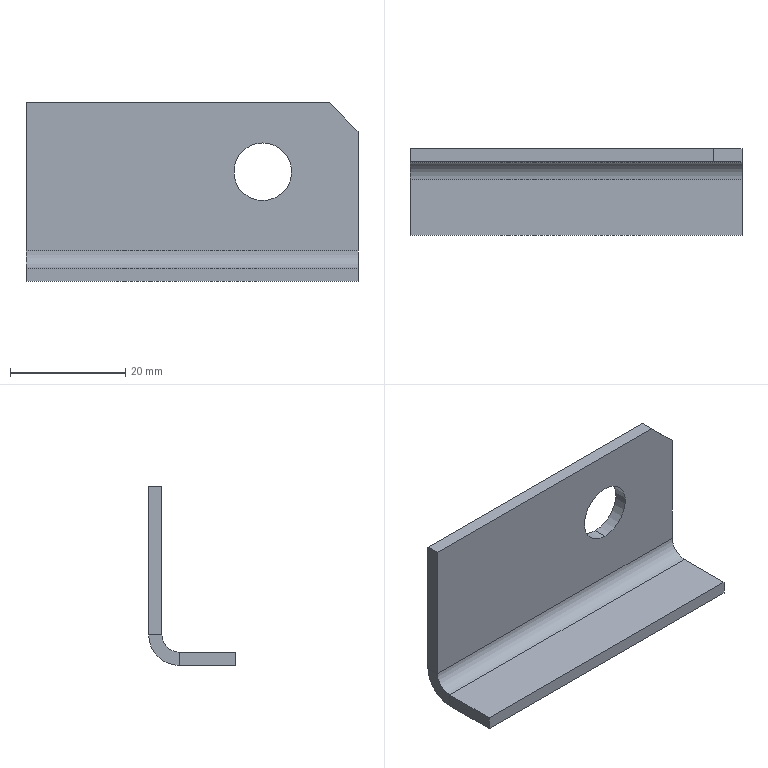Part | SolidWorks | features Chamfer 1, FlatPattern 1, ICE 1, SMBaseFlange 1, SheetMetal 1 | 1 solid | 17 faces | box 57.5 x 15 x 31 mm | volume 5334 mm3 | plane 13 | cylinder 4 | commonest cylinder face diameters 10 x2 6 x1 10.6 x1
STEP:
#1=CARTESIAN_POINT('',(12.25,15.,14.));
#2=VERTEX_POINT('',#1);
#3=CARTESIAN_POINT('',(12.25,15.,24.));
#4=VERTEX_POINT('',#3);
#5=CARTESIAN_POINT('',(12.25,15.,19.));
#6=DIRECTION('',(0.,1.,0.));
#7=DIRECTION('',(0.,0.,-1.));
#8=AXIS2_PLACEMENT_3D('',#5,#6,#7);
#9=CIRCLE('',#8,5.);
#10=EDGE_CURVE('',#2,#4,#9,.T.);
#11=ORIENTED_EDGE('',*,*,#10,.T.);
#12=CARTESIAN_POINT('',(12.25,12.7,24.));
#13=VERTEX_POINT('',#12);
#14=CARTESIAN_POINT('',(12.25,15.001,24.));
#15=DIRECTION('',(0.,-1.,0.));
#16=VECTOR('',#15,1000.);
#17=LINE('',#14,#16);
#18=EDGE_CURVE('',#4,#13,#17,.T.);
#19=ORIENTED_EDGE('',*,*,#18,.T.);
#20=CARTESIAN_POINT('',(12.25,12.7,14.));
#21=VERTEX_POINT('',#20);
#22=CARTESIAN_POINT('',(12.25,12.7,19.));
#23=DIRECTION('',(0.,-1.,0.));
#24=DIRECTION('',(0.,0.,-1.));
#25=AXIS2_PLACEMENT_3D('',#22,#23,#24);
#26=CIRCLE('',#25,5.);
#27=EDGE_CURVE('',#13,#21,#26,.T.);
#28=ORIENTED_EDGE('',*,*,#27,.T.);
#29=CARTESIAN_POINT('',(12.25,15.001,14.));
#30=DIRECTION('',(0.,-1.,0.));
#31=VECTOR('',#30,1000.);
#32=LINE('',#29,#31);
#33=EDGE_CURVE('',#2,#21,#32,.T.);
#34=ORIENTED_EDGE('',*,*,#33,.F.);
#35=EDGE_LOOP('',(#11,#19,#28,#34));
#36=FACE_OUTER_BOUND('',#35,.T.);
#37=CARTESIAN_POINT('',(12.25,15.001,19.));
#38=DIRECTION('',(0.,-1.,0.));
#39=DIRECTION('',(0.,0.,-1.));
#40=AXIS2_PLACEMENT_3D('',#37,#38,#39);
#41=CYLINDRICAL_SURFACE('',#40,5.);
#42=ADVANCED_FACE('',(#36),#41,.F.);
#43=CARTESIAN_POINT('',(28.75,9.7,0.));
#44=VERTEX_POINT('',#43);
#45=CARTESIAN_POINT('',(28.75,9.7,2.3));
#46=VERTEX_POINT('',#45);
#47=CARTESIAN_POINT('',(28.75,9.7,0.));
#48=DIRECTION('',(0.,0.,1.));
#49=VECTOR('',#48,1000.);
#50=LINE('',#47,#49);
#51=EDGE_CURVE('',#44,#46,#50,.T.);
#52=ORIENTED_EDGE('',*,*,#51,.F.);
#53=CARTESIAN_POINT('',(28.75,15.,5.3));
#54=VERTEX_POINT('',#53);
#55=CARTESIAN_POINT('',(28.75,9.7,5.3));
#56=DIRECTION('',(1.,0.,0.));
#57=DIRECTION('',(0.,0.,1.));
#58=AXIS2_PLACEMENT_3D('',#55,#56,#57);
#59=CIRCLE('',#58,5.3);
#60=EDGE_CURVE('',#44,#54,#59,.T.);
#61=ORIENTED_EDGE('',*,*,#60,.T.);
#62=CARTESIAN_POINT('',(28.75,12.7,5.3));
#63=VERTEX_POINT('',#62);
#64=CARTESIAN_POINT('',(28.75,12.7,5.3));
#65=DIRECTION('',(0.,1.,0.));
#66=VECTOR('',#65,1000.);
#67=LINE('',#64,#66);
#68=EDGE_CURVE('',#63,#54,#67,.T.);
#69=ORIENTED_EDGE('',*,*,#68,.F.);
#70=CARTESIAN_POINT('',(28.75,9.7,5.3));
#71=DIRECTION('',(1.,0.,0.));
#72=DIRECTION('',(0.,0.,-1.));
#73=AXIS2_PLACEMENT_3D('',#70,#71,#72);
#74=CIRCLE('',#73,3.);
#75=EDGE_CURVE('',#46,#63,#74,.T.);
#76=ORIENTED_EDGE('',*,*,#75,.F.);
#77=EDGE_LOOP('',(#52,#61,#69,#76));
#78=FACE_OUTER_BOUND('',#77,.T.);
#79=CARTESIAN_POINT('',(28.75,9.7,0.));
#80=DIRECTION('',(1.,0.,0.));
#81=DIRECTION('',(0.,0.,-1.));
#82=AXIS2_PLACEMENT_3D('',#79,#80,#81);
#83=PLANE('',#82);
#84=ADVANCED_FACE('',(#78),#83,.T.);
#85=CARTESIAN_POINT('',(28.75,0.,0.));
#86=VERTEX_POINT('',#85);
#87=CARTESIAN_POINT('',(28.75,0.,0.));
#88=DIRECTION('',(0.,1.,0.));
#89=VECTOR('',#88,1000.);
#90=LINE('',#87,#89);
#91=EDGE_CURVE('',#86,#44,#90,.T.);
#92=ORIENTED_EDGE('',*,*,#91,.T.);
#93=ORIENTED_EDGE('',*,*,#51,.T.);
#94=CARTESIAN_POINT('',(28.75,0.,2.3));
#95=VERTEX_POINT('',#94);
#96=CARTESIAN_POINT('',(28.75,0.,2.3));
#97=DIRECTION('',(0.,1.,0.));
#98=VECTOR('',#97,1000.);
#99=LINE('',#96,#98);
#100=EDGE_CURVE('',#95,#46,#99,.T.);
#101=ORIENTED_EDGE('',*,*,#100,.F.);
#102=CARTESIAN_POINT('',(28.75,0.,0.));
#103=DIRECTION('',(0.,0.,1.));
#104=VECTOR('',#103,1000.);
#105=LINE('',#102,#104);
#106=EDGE_CURVE('',#86,#95,#105,.T.);
#107=ORIENTED_EDGE('',*,*,#106,.F.);
#108=EDGE_LOOP('',(#92,#93,#101,#107));
#109=FACE_OUTER_BOUND('',#108,.T.);
#110=CARTESIAN_POINT('',(28.75,12.7,5.3));
#111=DIRECTION('',(1.,0.,0.));
#112=DIRECTION('',(0.,0.,-1.));
#113=AXIS2_PLACEMENT_3D('',#110,#111,#112);
#114=PLANE('',#113);
#115=ADVANCED_FACE('',(#109),#114,.T.);
#116=CARTESIAN_POINT('',(-28.75,15.,5.3));
#117=VERTEX_POINT('',#116);
#118=CARTESIAN_POINT('',(-28.75,12.7,5.3));
#119=VERTEX_POINT('',#118);
#120=CARTESIAN_POINT('',(-28.75,15.,5.3));
#121=DIRECTION('',(0.,-1.,0.));
#122=VECTOR('',#121,1000.);
#123=LINE('',#120,#122);
#124=EDGE_CURVE('',#117,#119,#123,.T.);
#125=ORIENTED_EDGE('',*,*,#124,.F.);
#126=CARTESIAN_POINT('',(-28.75,9.7,0.));
#127=VERTEX_POINT('',#126);
#128=CARTESIAN_POINT('',(-28.75,9.7,5.3));
#129=DIRECTION('',(1.,0.,0.));
#130=DIRECTION('',(0.,0.,1.));
#131=AXIS2_PLACEMENT_3D('',#128,#129,#130);
#132=CIRCLE('',#131,5.3);
#133=EDGE_CURVE('',#127,#117,#132,.T.);
#134=ORIENTED_EDGE('',*,*,#133,.F.);
#135=CARTESIAN_POINT('',(-28.75,9.7,2.3));
#136=VERTEX_POINT('',#135);
#137=CARTESIAN_POINT('',(-28.75,9.7,2.3));
#138=DIRECTION('',(0.,0.,-1.));
#139=VECTOR('',#138,1000.);
#140=LINE('',#137,#139);
#141=EDGE_CURVE('',#136,#127,#140,.T.);
#142=ORIENTED_EDGE('',*,*,#141,.F.);
#143=CARTESIAN_POINT('',(-28.75,9.7,5.3));
#144=DIRECTION('',(1.,0.,0.));
#145=DIRECTION('',(0.,0.,-1.));
#146=AXIS2_PLACEMENT_3D('',#143,#144,#145);
#147=CIRCLE('',#146,3.);
#148=EDGE_CURVE('',#136,#119,#147,.T.);
#149=ORIENTED_EDGE('',*,*,#148,.T.);
#150=EDGE_LOOP('',(#125,#134,#142,#149));
#151=FACE_OUTER_BOUND('',#150,.T.);
#152=CARTESIAN_POINT('',(-28.75,15.,5.3));
#153=DIRECTION('',(-1.,0.,0.));
#154=DIRECTION('',(0.,0.,1.));
#155=AXIS2_PLACEMENT_3D('',#152,#153,#154);
#156=PLANE('',#155);
#157=ADVANCED_FACE('',(#151),#156,.T.);
#158=CARTESIAN_POINT('',(-28.75,15.,31.));
#159=VERTEX_POINT('',#158);
#160=CARTESIAN_POINT('',(-28.75,15.,0.));
#161=DIRECTION('',(0.,0.,1.));
#162=VECTOR('',#161,1000.);
#163=LINE('',#160,#162);
#164=EDGE_CURVE('',#117,#159,#163,.T.);
#165=ORIENTED_EDGE('',*,*,#164,.F.);
#166=ORIENTED_EDGE('',*,*,#124,.T.);
#167=CARTESIAN_POINT('',(-28.75,12.7,31.));
#168=VERTEX_POINT('',#167);
#169=CARTESIAN_POINT('',(-28.75,12.7,0.));
#170=DIRECTION('',(0.,0.,1.));
#171=VECTOR('',#170,1000.);
#172=LINE('',#169,#171);
#173=EDGE_CURVE('',#119,#168,#172,.T.);
#174=ORIENTED_EDGE('',*,*,#173,.T.);
#175=CARTESIAN_POINT('',(-28.75,12.7,31.));
#176=DIRECTION('',(0.,1.,0.));
#177=VECTOR('',#176,1000.);
#178=LINE('',#175,#177);
#179=EDGE_CURVE('',#168,#159,#178,.T.);
#180=ORIENTED_EDGE('',*,*,#179,.T.);
#181=EDGE_LOOP('',(#165,#166,#174,#180));
#182=FACE_OUTER_BOUND('',#181,.T.);
#183=CARTESIAN_POINT('',(-28.75,9.7,2.3));
#184=DIRECTION('',(-1.,0.,0.));
#185=DIRECTION('',(0.,0.,1.));
#186=AXIS2_PLACEMENT_3D('',#183,#184,#185);
#187=PLANE('',#186);
#188=ADVANCED_FACE('',(#182),#187,.T.);
#189=ORIENTED_EDGE('',*,*,#10,.F.);
#190=CARTESIAN_POINT('',(12.25,15.,19.));
#191=DIRECTION('',(0.,1.,0.));
#192=DIRECTION('',(0.,0.,-1.));
#193=AXIS2_PLACEMENT_3D('',#190,#191,#192);
#194=CIRCLE('',#193,5.);
#195=EDGE_CURVE('',#4,#2,#194,.T.);
#196=ORIENTED_EDGE('',*,*,#195,.F.);
#197=EDGE_LOOP('',(#189,#196));
#198=FACE_BOUND('',#197,.T.);
#199=CARTESIAN_POINT('',(23.75,15.,31.));
#200=VERTEX_POINT('',#199);
#201=CARTESIAN_POINT('',(28.75,15.,31.));
#202=DIRECTION('',(-1.,0.,0.));
#203=VECTOR('',#202,1000.);
#204=LINE('',#201,#203);
#205=EDGE_CURVE('',#200,#159,#204,.T.);
#206=ORIENTED_EDGE('',*,*,#205,.F.);
#207=CARTESIAN_POINT('',(28.75,15.,26.));
#208=VERTEX_POINT('',#207);
#209=CARTESIAN_POINT('',(23.75,15.,31.));
#210=DIRECTION('',(0.7071,0.,-0.7071));
#211=VECTOR('',#210,1000.);
#212=LINE('',#209,#211);
#213=EDGE_CURVE('',#200,#208,#212,.T.);
#214=ORIENTED_EDGE('',*,*,#213,.T.);
#215=CARTESIAN_POINT('',(28.75,15.,0.));
#216=DIRECTION('',(0.,0.,1.));
#217=VECTOR('',#216,1000.);
#218=LINE('',#215,#217);
#219=EDGE_CURVE('',#54,#208,#218,.T.);
#220=ORIENTED_EDGE('',*,*,#219,.F.);
#221=CARTESIAN_POINT('',(28.75,15.,5.3));
#222=DIRECTION('',(-1.,0.,0.));
#223=VECTOR('',#222,1000.);
#224=LINE('',#221,#223);
#225=EDGE_CURVE('',#54,#117,#224,.T.);
#226=ORIENTED_EDGE('',*,*,#225,.T.);
#227=ORIENTED_EDGE('',*,*,#164,.T.);
#228=EDGE_LOOP('',(#206,#214,#220,#226,#227));
#229=FACE_OUTER_BOUND('',#228,.T.);
#230=CARTESIAN_POINT('',(28.75,15.,0.));
#231=DIRECTION('',(0.,-1.,0.));
#232=DIRECTION('',(0.,0.,-1.));
#233=AXIS2_PLACEMENT_3D('',#230,#231,#232);
#234=PLANE('',#233);
#235=ADVANCED_FACE('',(#198,#229),#234,.F.);
#236=CARTESIAN_POINT('',(23.75,12.7,31.));
#237=VERTEX_POINT('',#236);
#238=CARTESIAN_POINT('',(28.75,12.7,31.));
#239=DIRECTION('',(-1.,0.,0.));
#240=VECTOR('',#239,1000.);
#241=LINE('',#238,#240);
#242=EDGE_CURVE('',#237,#168,#241,.T.);
#243=ORIENTED_EDGE('',*,*,#242,.F.);
#244=CARTESIAN_POINT('',(23.75,12.7,31.));
#245=DIRECTION('',(0.,1.,0.));
#246=VECTOR('',#245,1000.);
#247=LINE('',#244,#246);
#248=EDGE_CURVE('',#237,#200,#247,.T.);
#249=ORIENTED_EDGE('',*,*,#248,.T.);
#250=ORIENTED_EDGE('',*,*,#205,.T.);
#251=ORIENTED_EDGE('',*,*,#179,.F.);
#252=EDGE_LOOP('',(#243,#249,#250,#251));
#253=FACE_OUTER_BOUND('',#252,.T.);
#254=CARTESIAN_POINT('',(28.75,12.7,31.));
#255=DIRECTION('',(0.,0.,1.));
#256=DIRECTION('',(1.,0.,0.));
#257=AXIS2_PLACEMENT_3D('',#254,#255,#256);
#258=PLANE('',#257);
#259=ADVANCED_FACE('',(#253),#258,.T.);
#260=CARTESIAN_POINT('',(12.25,12.7,19.));
#261=DIRECTION('',(0.,-1.,0.));
#262=DIRECTION('',(0.,0.,-1.));
#263=AXIS2_PLACEMENT_3D('',#260,#261,#262);
#264=CIRCLE('',#263,5.);
#265=EDGE_CURVE('',#21,#13,#264,.T.);
#266=ORIENTED_EDGE('',*,*,#265,.F.);
#267=ORIENTED_EDGE('',*,*,#27,.F.);
#268=EDGE_LOOP('',(#266,#267));
#269=FACE_BOUND('',#268,.T.);
#270=CARTESIAN_POINT('',(28.75,12.7,26.));
#271=VERTEX_POINT('',#270);
#272=CARTESIAN_POINT('',(28.75,12.7,0.));
#273=DIRECTION('',(0.,0.,1.));
#274=VECTOR('',#273,1000.);
#275=LINE('',#272,#274);
#276=EDGE_CURVE('',#63,#271,#275,.T.);
#277=ORIENTED_EDGE('',*,*,#276,.T.);
#278=CARTESIAN_POINT('',(41.75,12.7,13.));
#279=DIRECTION('',(-0.7071,0.,0.7071));
#280=VECTOR('',#279,1000.);
#281=LINE('',#278,#280);
#282=EDGE_CURVE('',#271,#237,#281,.T.);
#283=ORIENTED_EDGE('',*,*,#282,.T.);
#284=ORIENTED_EDGE('',*,*,#242,.T.);
#285=ORIENTED_EDGE('',*,*,#173,.F.);
#286=CARTESIAN_POINT('',(28.75,12.7,5.3));
#287=DIRECTION('',(-1.,0.,0.));
#288=VECTOR('',#287,1000.);
#289=LINE('',#286,#288);
#290=EDGE_CURVE('',#63,#119,#289,.T.);
#291=ORIENTED_EDGE('',*,*,#290,.F.);
#292=EDGE_LOOP('',(#277,#283,#284,#285,#291));
#293=FACE_OUTER_BOUND('',#292,.T.);
#294=CARTESIAN_POINT('',(28.75,12.7,0.));
#295=DIRECTION('',(0.,-1.,0.));
#296=DIRECTION('',(0.,0.,-1.));
#297=AXIS2_PLACEMENT_3D('',#294,#295,#296);
#298=PLANE('',#297);
#299=ADVANCED_FACE('',(#269,#293),#298,.T.);
#300=ORIENTED_EDGE('',*,*,#148,.F.);
#301=CARTESIAN_POINT('',(28.75,9.7,2.3));
#302=DIRECTION('',(-1.,0.,0.));
#303=VECTOR('',#302,1000.);
#304=LINE('',#301,#303);
#305=EDGE_CURVE('',#46,#136,#304,.T.);
#306=ORIENTED_EDGE('',*,*,#305,.F.);
#307=ORIENTED_EDGE('',*,*,#75,.T.);
#308=ORIENTED_EDGE('',*,*,#290,.T.);
#309=EDGE_LOOP('',(#300,#306,#307,#308));
#310=FACE_OUTER_BOUND('',#309,.T.);
#311=CARTESIAN_POINT('',(28.75,9.7,5.3));
#312=DIRECTION('',(-1.,0.,0.));
#313=DIRECTION('',(0.,0.,1.));
#314=AXIS2_PLACEMENT_3D('',#311,#312,#313);
#315=CYLINDRICAL_SURFACE('',#314,3.);
#316=ADVANCED_FACE('',(#310),#315,.F.);
#317=CARTESIAN_POINT('',(-28.75,0.,2.3));
#318=VERTEX_POINT('',#317);
#319=CARTESIAN_POINT('',(-28.75,0.,2.3));
#320=DIRECTION('',(0.,1.,0.));
#321=VECTOR('',#320,1000.);
#322=LINE('',#319,#321);
#323=EDGE_CURVE('',#318,#136,#322,.T.);
#324=ORIENTED_EDGE('',*,*,#323,.F.);
#325=CARTESIAN_POINT('',(28.75,0.,2.3));
#326=DIRECTION('',(-1.,0.,0.));
#327=VECTOR('',#326,1000.);
#328=LINE('',#325,#327);
#329=EDGE_CURVE('',#95,#318,#328,.T.);
#330=ORIENTED_EDGE('',*,*,#329,.F.);
#331=ORIENTED_EDGE('',*,*,#100,.T.);
#332=ORIENTED_EDGE('',*,*,#305,.T.);
#333=EDGE_LOOP('',(#324,#330,#331,#332));
#334=FACE_OUTER_BOUND('',#333,.T.);
#335=CARTESIAN_POINT('',(28.75,0.,2.3));
#336=DIRECTION('',(0.,0.,1.));
#337=DIRECTION('',(1.,0.,0.));
#338=AXIS2_PLACEMENT_3D('',#335,#336,#337);
#339=PLANE('',#338);
#340=ADVANCED_FACE('',(#334),#339,.T.);
#341=CARTESIAN_POINT('',(-28.75,0.,0.));
#342=VERTEX_POINT('',#341);
#343=CARTESIAN_POINT('',(-28.75,0.,0.));
#344=DIRECTION('',(0.,0.,1.));
#345=VECTOR('',#344,1000.);
#346=LINE('',#343,#345);
#347=EDGE_CURVE('',#342,#318,#346,.T.);
#348=ORIENTED_EDGE('',*,*,#347,.F.);
#349=CARTESIAN_POINT('',(28.75,0.,0.));
#350=DIRECTION('',(-1.,0.,0.));
#351=VECTOR('',#350,1000.);
#352=LINE('',#349,#351);
#353=EDGE_CURVE('',#86,#342,#352,.T.);
#354=ORIENTED_EDGE('',*,*,#353,.F.);
#355=ORIENTED_EDGE('',*,*,#106,.T.);
#356=ORIENTED_EDGE('',*,*,#329,.T.);
#357=EDGE_LOOP('',(#348,#354,#355,#356));
#358=FACE_OUTER_BOUND('',#357,.T.);
#359=CARTESIAN_POINT('',(28.75,0.,0.));
#360=DIRECTION('',(0.,-1.,0.));
#361=DIRECTION('',(0.,0.,-1.));
#362=AXIS2_PLACEMENT_3D('',#359,#360,#361);
#363=PLANE('',#362);
#364=ADVANCED_FACE('',(#358),#363,.T.);
#365=CARTESIAN_POINT('',(-28.75,0.,0.));
#366=DIRECTION('',(0.,1.,0.));
#367=VECTOR('',#366,1000.);
#368=LINE('',#365,#367);
#369=EDGE_CURVE('',#342,#127,#368,.T.);
#370=ORIENTED_EDGE('',*,*,#369,.T.);
#371=CARTESIAN_POINT('',(28.75,9.7,0.));
#372=DIRECTION('',(-1.,0.,0.));
#373=VECTOR('',#372,1000.);
#374=LINE('',#371,#373);
#375=EDGE_CURVE('',#44,#127,#374,.T.);
#376=ORIENTED_EDGE('',*,*,#375,.F.);
#377=ORIENTED_EDGE('',*,*,#91,.F.);
#378=ORIENTED_EDGE('',*,*,#353,.T.);
#379=EDGE_LOOP('',(#370,#376,#377,#378));
#380=FACE_OUTER_BOUND('',#379,.T.);
#381=CARTESIAN_POINT('',(28.75,0.,0.));
#382=DIRECTION('',(0.,0.,1.));
#383=DIRECTION('',(1.,0.,0.));
#384=AXIS2_PLACEMENT_3D('',#381,#382,#383);
#385=PLANE('',#384);
#386=ADVANCED_FACE('',(#380),#385,.F.);
#387=ORIENTED_EDGE('',*,*,#133,.T.);
#388=ORIENTED_EDGE('',*,*,#225,.F.);
#389=ORIENTED_EDGE('',*,*,#60,.F.);
#390=ORIENTED_EDGE('',*,*,#375,.T.);
#391=EDGE_LOOP('',(#387,#388,#389,#390));
#392=FACE_OUTER_BOUND('',#391,.T.);
#393=CARTESIAN_POINT('',(28.75,9.7,5.3));
#394=DIRECTION('',(-1.,0.,0.));
#395=DIRECTION('',(0.,0.,1.));
#396=AXIS2_PLACEMENT_3D('',#393,#394,#395);
#397=CYLINDRICAL_SURFACE('',#396,5.3);
#398=ADVANCED_FACE('',(#392),#397,.T.);
#399=ORIENTED_EDGE('',*,*,#219,.T.);
#400=CARTESIAN_POINT('',(28.75,9.7,26.));
#401=DIRECTION('',(0.,-1.,0.));
#402=VECTOR('',#401,1000.);
#403=LINE('',#400,#402);
#404=EDGE_CURVE('',#208,#271,#403,.T.);
#405=ORIENTED_EDGE('',*,*,#404,.T.);
#406=ORIENTED_EDGE('',*,*,#276,.F.);
#407=ORIENTED_EDGE('',*,*,#68,.T.);
#408=EDGE_LOOP('',(#399,#405,#406,#407));
#409=FACE_OUTER_BOUND('',#408,.T.);
#410=CARTESIAN_POINT('',(28.75,9.7,5.3));
#411=DIRECTION('',(1.,0.,0.));
#412=DIRECTION('',(0.,0.,-1.));
#413=AXIS2_PLACEMENT_3D('',#410,#411,#412);
#414=PLANE('',#413);
#415=ADVANCED_FACE('',(#409),#414,.T.);
#416=ORIENTED_EDGE('',*,*,#323,.T.);
#417=ORIENTED_EDGE('',*,*,#141,.T.);
#418=ORIENTED_EDGE('',*,*,#369,.F.);
#419=ORIENTED_EDGE('',*,*,#347,.T.);
#420=EDGE_LOOP('',(#416,#417,#418,#419));
#421=FACE_OUTER_BOUND('',#420,.T.);
#422=CARTESIAN_POINT('',(-28.75,9.7,5.3));
#423=DIRECTION('',(1.,0.,0.));
#424=DIRECTION('',(0.,0.,-1.));
#425=AXIS2_PLACEMENT_3D('',#422,#423,#424);
#426=PLANE('',#425);
#427=ADVANCED_FACE('',(#421),#426,.F.);
#428=ORIENTED_EDGE('',*,*,#18,.F.);
#429=ORIENTED_EDGE('',*,*,#195,.T.);
#430=ORIENTED_EDGE('',*,*,#33,.T.);
#431=ORIENTED_EDGE('',*,*,#265,.T.);
#432=EDGE_LOOP('',(#428,#429,#430,#431));
#433=FACE_OUTER_BOUND('',#432,.T.);
#434=CARTESIAN_POINT('',(12.25,15.001,19.));
#435=DIRECTION('',(0.,-1.,0.));
#436=DIRECTION('',(0.,0.,-1.));
#437=AXIS2_PLACEMENT_3D('',#434,#435,#436);
#438=CYLINDRICAL_SURFACE('',#437,5.);
#439=ADVANCED_FACE('',(#433),#438,.F.);
#440=ORIENTED_EDGE('',*,*,#282,.F.);
#441=ORIENTED_EDGE('',*,*,#404,.F.);
#442=ORIENTED_EDGE('',*,*,#213,.F.);
#443=ORIENTED_EDGE('',*,*,#248,.F.);
#444=EDGE_LOOP('',(#440,#441,#442,#443));
#445=FACE_OUTER_BOUND('',#444,.T.);
#446=CARTESIAN_POINT('',(23.75,12.7,31.));
#447=DIRECTION('',(-0.7071,0.,-0.7071));
#448=DIRECTION('',(0.,1.,0.));
#449=AXIS2_PLACEMENT_3D('',#446,#447,#448);
#450=PLANE('',#449);
#451=ADVANCED_FACE('',(#445),#450,.F.);
#452=CLOSED_SHELL('',(#42,#84,#115,#157,#188,#235,#259,#299,#316,#340,#364,#386,#398,#415,#427,#439,#451));
#453=MANIFOLD_SOLID_BREP('',#452);
#454=CARTESIAN_POINT('',(0.,0.,0.));
#455=DIRECTION('',(0.,0.,1.));
#456=DIRECTION('',(1.,0.,0.));
#457=AXIS2_PLACEMENT_3D('',#454,#455,#456);
#458=(LENGTH_UNIT()NAMED_UNIT(*)SI_UNIT(.MILLI.,.METRE.));
#459=UNCERTAINTY_MEASURE_WITH_UNIT(LENGTH_MEASURE(0.00001),#458,'','');
#460=(NAMED_UNIT(*)PLANE_ANGLE_UNIT()SI_UNIT($,.RADIAN.));
#461=(NAMED_UNIT(*)SI_UNIT($,.STERADIAN.)SOLID_ANGLE_UNIT());
#462=(GEOMETRIC_REPRESENTATION_CONTEXT(3)GLOBAL_UNCERTAINTY_ASSIGNED_CONTEXT((#459))GLOBAL_UNIT_ASSIGNED_CONTEXT((#458,#460,#461))REPRESENTATION_CONTEXT('',''));
#463=ADVANCED_BREP_SHAPE_REPRESENTATION('',(#453,#457),#462);